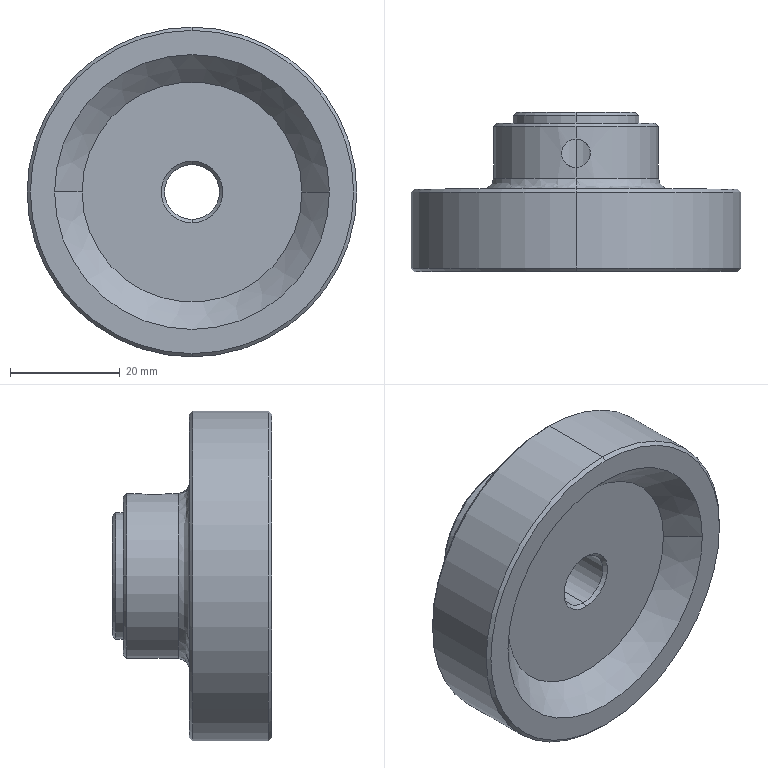Part | SolidWorks | features BaseBody 1 | 1 solid | 31 faces | box 60 x 29 x 60 mm | volume 41614 mm3 | cone 14 | cylinder 10 | plane 5 | spline 2 | commonest cylinder face diameters 5.2 x2 10 x2 23 x2 30 x2 60 x2
STEP:
#1=CARTESIAN_POINT('',(0.,10.655,-15.));
#2=VERTEX_POINT('',#1);
#3=CARTESIAN_POINT('',(0.,10.655,15.));
#4=VERTEX_POINT('',#3);
#5=CARTESIAN_POINT('',(0.,10.655,0.));
#6=DIRECTION('',(0.,1.,0.));
#7=DIRECTION('',(0.,0.,1.));
#8=AXIS2_PLACEMENT_3D('',#5,#6,#7);
#9=CIRCLE('',#8,15.);
#10=EDGE_CURVE('',#2,#4,#9,.T.);
#11=ORIENTED_EDGE('',*,*,#10,.F.);
#12=CARTESIAN_POINT('',(0.,8.655,-17.));
#13=VERTEX_POINT('',#12);
#14=CARTESIAN_POINT('',(0.,10.655,-17.));
#15=DIRECTION('',(1.,0.,0.));
#16=DIRECTION('',(0.,0.,-1.));
#17=AXIS2_PLACEMENT_3D('',#14,#15,#16);
#18=CIRCLE('',#17,2.);
#19=EDGE_CURVE('',#2,#13,#18,.T.);
#20=ORIENTED_EDGE('',*,*,#19,.T.);
#21=CARTESIAN_POINT('',(0.,8.655,17.));
#22=VERTEX_POINT('',#21);
#23=CARTESIAN_POINT('',(0.,8.655,17.));
#24=CARTESIAN_POINT('',(-0.5198,8.655,17.));
#25=CARTESIAN_POINT('',(-1.296,8.655,16.965));
#26=CARTESIAN_POINT('',(-2.197,8.655,16.861));
#27=CARTESIAN_POINT('',(-2.646,8.655,16.794));
#28=CARTESIAN_POINT('',(-2.87,8.655,16.756));
#29=CARTESIAN_POINT('',(-2.966,8.655,16.739));
#30=CARTESIAN_POINT('',(-3.029,8.655,16.728));
#31=CARTESIAN_POINT('',(-3.059,8.655,16.722));
#32=CARTESIAN_POINT('',(-3.635,8.655,16.616));
#33=CARTESIAN_POINT('',(-4.437,8.655,16.427));
#34=CARTESIAN_POINT('',(-5.354,8.655,16.139));
#35=CARTESIAN_POINT('',(-5.807,8.655,15.978));
#36=CARTESIAN_POINT('',(-6.033,8.655,15.894));
#37=CARTESIAN_POINT('',(-6.129,8.655,15.857));
#38=CARTESIAN_POINT('',(-6.193,8.655,15.832));
#39=CARTESIAN_POINT('',(-6.224,8.655,15.82));
#40=CARTESIAN_POINT('',(-6.792,8.655,15.595));
#41=CARTESIAN_POINT('',(-7.573,8.655,15.239));
#42=CARTESIAN_POINT('',(-8.449,8.655,14.757));
#43=CARTESIAN_POINT('',(-8.879,8.655,14.498));
#44=CARTESIAN_POINT('',(-9.061,8.655,14.384));
#45=CARTESIAN_POINT('',(-9.182,8.655,14.307));
#46=CARTESIAN_POINT('',(-9.241,8.655,14.269));
#47=CARTESIAN_POINT('',(-10.285,8.655,13.587));
#48=CARTESIAN_POINT('',(-11.191,8.655,12.85));
#49=CARTESIAN_POINT('',(-12.436,8.655,11.606));
#50=CARTESIAN_POINT('',(-13.023,8.655,10.955));
#51=CARTESIAN_POINT('',(-13.646,8.655,10.146));
#52=CARTESIAN_POINT('',(-13.943,8.655,9.728));
#53=CARTESIAN_POINT('',(-14.066,8.655,9.547));
#54=CARTESIAN_POINT('',(-14.148,8.655,9.425));
#55=CARTESIAN_POINT('',(-14.19,8.655,9.363));
#56=CARTESIAN_POINT('',(-14.543,8.655,8.822));
#57=CARTESIAN_POINT('',(-14.976,8.655,8.081));
#58=CARTESIAN_POINT('',(-15.414,8.655,7.181));
#59=CARTESIAN_POINT('',(-15.616,8.655,6.722));
#60=CARTESIAN_POINT('',(-15.712,8.655,6.491));
#61=CARTESIAN_POINT('',(-15.753,8.655,6.391));
#62=CARTESIAN_POINT('',(-15.78,8.655,6.324));
#63=CARTESIAN_POINT('',(-15.794,8.655,6.29));
#64=CARTESIAN_POINT('',(-16.009,8.655,5.745));
#65=CARTESIAN_POINT('',(-16.275,8.655,4.965));
#66=CARTESIAN_POINT('',(-16.518,8.655,4.036));
#67=CARTESIAN_POINT('',(-16.623,8.655,3.566));
#68=CARTESIAN_POINT('',(-16.671,8.655,3.33));
#69=CARTESIAN_POINT('',(-16.691,8.655,3.229));
#70=CARTESIAN_POINT('',(-16.704,8.655,3.161));
#71=CARTESIAN_POINT('',(-16.71,8.655,3.125));
#72=CARTESIAN_POINT('',(-16.905,8.655,2.071));
#73=CARTESIAN_POINT('',(-17.,8.655,1.039));
#74=CARTESIAN_POINT('',(-17.,8.655,-0.5197));
#75=CARTESIAN_POINT('',(-16.965,8.655,-1.296));
#76=CARTESIAN_POINT('',(-16.861,8.655,-2.197));
#77=CARTESIAN_POINT('',(-16.794,8.655,-2.645));
#78=CARTESIAN_POINT('',(-16.756,8.655,-2.87));
#79=CARTESIAN_POINT('',(-16.739,8.655,-2.965));
#80=CARTESIAN_POINT('',(-16.728,8.655,-3.029));
#81=CARTESIAN_POINT('',(-16.722,8.655,-3.059));
#82=CARTESIAN_POINT('',(-16.616,8.655,-3.635));
#83=CARTESIAN_POINT('',(-16.427,8.655,-4.437));
#84=CARTESIAN_POINT('',(-16.139,8.655,-5.354));
#85=CARTESIAN_POINT('',(-15.978,8.655,-5.807));
#86=CARTESIAN_POINT('',(-15.894,8.655,-6.033));
#87=CARTESIAN_POINT('',(-15.857,8.655,-6.129));
#88=CARTESIAN_POINT('',(-15.832,8.655,-6.193));
#89=CARTESIAN_POINT('',(-15.82,8.655,-6.224));
#90=CARTESIAN_POINT('',(-15.595,8.655,-6.792));
#91=CARTESIAN_POINT('',(-15.239,8.655,-7.573));
#92=CARTESIAN_POINT('',(-14.757,8.655,-8.449));
#93=CARTESIAN_POINT('',(-14.498,8.655,-8.879));
#94=CARTESIAN_POINT('',(-14.384,8.655,-9.061));
#95=CARTESIAN_POINT('',(-14.307,8.655,-9.182));
#96=CARTESIAN_POINT('',(-14.269,8.655,-9.241));
#97=CARTESIAN_POINT('',(-13.587,8.655,-10.285));
#98=CARTESIAN_POINT('',(-12.85,8.655,-11.191));
#99=CARTESIAN_POINT('',(-11.606,8.655,-12.436));
#100=CARTESIAN_POINT('',(-10.955,8.655,-13.023));
#101=CARTESIAN_POINT('',(-10.146,8.655,-13.646));
#102=CARTESIAN_POINT('',(-9.728,8.655,-13.943));
#103=CARTESIAN_POINT('',(-9.547,8.655,-14.066));
#104=CARTESIAN_POINT('',(-9.425,8.655,-14.148));
#105=CARTESIAN_POINT('',(-9.363,8.655,-14.19));
#106=CARTESIAN_POINT('',(-8.822,8.655,-14.543));
#107=CARTESIAN_POINT('',(-8.081,8.655,-14.976));
#108=CARTESIAN_POINT('',(-7.181,8.655,-15.414));
#109=CARTESIAN_POINT('',(-6.722,8.655,-15.616));
#110=CARTESIAN_POINT('',(-6.491,8.655,-15.712));
#111=CARTESIAN_POINT('',(-6.391,8.655,-15.753));
#112=CARTESIAN_POINT('',(-6.324,8.655,-15.78));
#113=CARTESIAN_POINT('',(-6.29,8.655,-15.794));
#114=CARTESIAN_POINT('',(-5.745,8.655,-16.009));
#115=CARTESIAN_POINT('',(-4.965,8.655,-16.275));
#116=CARTESIAN_POINT('',(-4.036,8.655,-16.518));
#117=CARTESIAN_POINT('',(-3.566,8.655,-16.623));
#118=CARTESIAN_POINT('',(-3.33,8.655,-16.671));
#119=CARTESIAN_POINT('',(-3.229,8.655,-16.691));
#120=CARTESIAN_POINT('',(-3.161,8.655,-16.704));
#121=CARTESIAN_POINT('',(-3.125,8.655,-16.71));
#122=CARTESIAN_POINT('',(-2.071,8.655,-16.905));
#123=CARTESIAN_POINT('',(-1.04,8.655,-17.));
#124=CARTESIAN_POINT('',(0.,8.655,-17.));
#125=B_SPLINE_CURVE_WITH_KNOTS('',3,(#23,#24,#25,#26,#27,#28,#29,#30,#31,#32,#33,#34,#35,#36,#37,#38,#39,#40,#41,#42,#43,#44,#45,#46,#47,#48,#49,#50,#51,#52,#53,#54,#55,#56,#57,#58,#59,#60,#61,#62,#63,#64,#65,#66,#67,#68,#69,#70,#71,#72,#73,#74,#75,#76,#77,#78,#79,#80,#81,#82,#83,#84,#85,#86,#87,#88,#89,#90,#91,#92,#93,#94,#95,#96,#97,#98,#99,#100,#101,#102,#103,#104,#105,#106,#107,#108,#109,#110,#111,#112,#113,#114,#115,#116,#117,#118,#119,#120,#121,#122,#123,#124),.UNSPECIFIED.,.F.,.F.,(4,1,1,1,1,2,2,1,1,1,1,2,2,1,1,1,2,2,2,1,1,1,2,2,1,1,1,1,2,2,1,1,1,1,2,2,2,1,1,1,1,2,2,1,1,1,1,2,2,1,1,1,2,2,2,1,1,1,2,2,1,1,1,1,2,2,1,1,1,1,2,2,4),(0.,0.03125,0.04688,0.05469,0.05859,0.06055,0.0625,0.09375,0.1094,0.1172,0.1211,0.123,0.125,0.1562,0.1719,0.1797,0.1836,0.1875,0.25,0.2812,0.2969,0.3047,0.3086,0.3125,0.3437,0.3594,0.3672,0.3711,0.373,0.375,0.4062,0.4219,0.4297,0.4336,0.4355,0.4375,0.5,0.5313,0.5469,0.5547,0.5586,0.5605,0.5625,0.5938,0.6094,0.6172,0.6211,0.623,0.625,0.6563,0.6719,0.6797,0.6836,0.6875,0.75,0.7813,0.7969,0.8047,0.8086,0.8125,0.8438,0.8594,0.8672,0.8711,0.873,0.875,0.9063,0.9219,0.9297,0.9336,0.9355,0.9375,1.),.UNSPECIFIED.);
#126=EDGE_CURVE('',#22,#13,#125,.T.);
#127=ORIENTED_EDGE('',*,*,#126,.F.);
#128=CARTESIAN_POINT('',(0.,10.655,17.));
#129=DIRECTION('',(-1.,0.,0.));
#130=DIRECTION('',(0.,0.,1.));
#131=AXIS2_PLACEMENT_3D('',#128,#129,#130);
#132=CIRCLE('',#131,2.);
#133=EDGE_CURVE('',#4,#22,#132,.T.);
#134=ORIENTED_EDGE('',*,*,#133,.F.);
#135=EDGE_LOOP('',(#11,#20,#127,#134));
#136=FACE_OUTER_BOUND('',#135,.T.);
#137=CARTESIAN_POINT('',(0.,10.655,15.));
#138=CARTESIAN_POINT('',(-30.,10.655,15.));
#139=CARTESIAN_POINT('',(-30.,10.655,-15.));
#140=CARTESIAN_POINT('',(0.,10.655,-15.));
#141=CARTESIAN_POINT('',(0.,9.484,15.));
#142=CARTESIAN_POINT('',(-30.,9.484,15.));
#143=CARTESIAN_POINT('',(-30.,9.484,-15.));
#144=CARTESIAN_POINT('',(0.,9.484,-15.));
#145=CARTESIAN_POINT('',(0.,8.655,15.828));
#146=CARTESIAN_POINT('',(-31.657,8.655,15.828));
#147=CARTESIAN_POINT('',(-31.657,8.655,-15.828));
#148=CARTESIAN_POINT('',(0.,8.655,-15.828));
#149=CARTESIAN_POINT('',(0.,8.655,17.));
#150=CARTESIAN_POINT('',(-34.,8.655,17.));
#151=CARTESIAN_POINT('',(-34.,8.655,-17.));
#152=CARTESIAN_POINT('',(0.,8.655,-17.));
#153=(BOUNDED_SURFACE()B_SPLINE_SURFACE(3,3,((#137,#138,#139,#140),(#141,#142,#143,#144),(#145,#146,#147,#148),(#149,#150,#151,#152)),.UNSPECIFIED.,.F.,.F.,.F.)B_SPLINE_SURFACE_WITH_KNOTS((4,4),(4,4),(0.,1.),(0.,1.),.UNSPECIFIED.)GEOMETRIC_REPRESENTATION_ITEM()RATIONAL_B_SPLINE_SURFACE(((1.,0.3333,0.3333,1.),(0.8047,0.2682,0.2682,0.8047),(0.8047,0.2682,0.2682,0.8047),(1.,0.3333,0.3333,1.)))REPRESENTATION_ITEM('')SURFACE());
#154=ADVANCED_FACE('',(#136),#153,.F.);
#155=CARTESIAN_POINT('',(0.,8.655,29.4));
#156=VERTEX_POINT('',#155);
#157=CARTESIAN_POINT('',(0.,8.655,-29.4));
#158=VERTEX_POINT('',#157);
#159=CARTESIAN_POINT('',(0.,8.655,0.));
#160=DIRECTION('',(0.,1.,0.));
#161=DIRECTION('',(0.,0.,-1.));
#162=AXIS2_PLACEMENT_3D('',#159,#160,#161);
#163=CIRCLE('',#162,29.4);
#164=EDGE_CURVE('',#156,#158,#163,.T.);
#165=ORIENTED_EDGE('',*,*,#164,.F.);
#166=CARTESIAN_POINT('',(0.,8.055,30.));
#167=VERTEX_POINT('',#166);
#168=CARTESIAN_POINT('',(0.,8.055,30.));
#169=DIRECTION('',(0.,-0.7071,0.7071));
#170=VECTOR('',#169,1000.);
#171=LINE('',#168,#170);
#172=EDGE_CURVE('',#156,#167,#171,.T.);
#173=ORIENTED_EDGE('',*,*,#172,.T.);
#174=CARTESIAN_POINT('',(0.,8.055,-30.));
#175=VERTEX_POINT('',#174);
#176=CARTESIAN_POINT('',(0.,8.055,0.));
#177=DIRECTION('',(0.,1.,0.));
#178=DIRECTION('',(0.,0.,1.));
#179=AXIS2_PLACEMENT_3D('',#176,#177,#178);
#180=CIRCLE('',#179,30.);
#181=EDGE_CURVE('',#167,#175,#180,.T.);
#182=ORIENTED_EDGE('',*,*,#181,.T.);
#183=CARTESIAN_POINT('',(0.,8.055,-30.));
#184=DIRECTION('',(0.,-0.7071,-0.7071));
#185=VECTOR('',#184,1000.);
#186=LINE('',#183,#185);
#187=EDGE_CURVE('',#158,#175,#186,.T.);
#188=ORIENTED_EDGE('',*,*,#187,.F.);
#189=EDGE_LOOP('',(#165,#173,#182,#188));
#190=FACE_OUTER_BOUND('',#189,.T.);
#191=CARTESIAN_POINT('',(0.,8.055,0.));
#192=DIRECTION('',(0.,-1.,0.));
#193=DIRECTION('',(0.,0.,-1.));
#194=AXIS2_PLACEMENT_3D('',#191,#192,#193);
#195=CONICAL_SURFACE('',#194,30.,0.7854);
#196=ADVANCED_FACE('',(#190),#195,.T.);
#197=CARTESIAN_POINT('',(15.,20.055,0.));
#198=VERTEX_POINT('',#197);
#199=CARTESIAN_POINT('',(0.,20.055,15.));
#200=VERTEX_POINT('',#199);
#201=CARTESIAN_POINT('',(0.,20.055,0.));
#202=DIRECTION('',(0.,-1.,0.));
#203=DIRECTION('',(0.,0.,-1.));
#204=AXIS2_PLACEMENT_3D('',#201,#202,#203);
#205=CIRCLE('',#204,15.);
#206=EDGE_CURVE('',#198,#200,#205,.T.);
#207=ORIENTED_EDGE('',*,*,#206,.T.);
#208=CARTESIAN_POINT('',(0.,17.755,15.));
#209=VERTEX_POINT('',#208);
#210=CARTESIAN_POINT('',(0.,0.,15.));
#211=DIRECTION('',(0.,-1.,0.));
#212=VECTOR('',#211,1000.);
#213=LINE('',#210,#212);
#214=EDGE_CURVE('',#200,#209,#213,.T.);
#215=ORIENTED_EDGE('',*,*,#214,.T.);
#216=CARTESIAN_POINT('',(2.6,15.155,14.773));
#217=VERTEX_POINT('',#216);
#218=CARTESIAN_POINT('',(0.,17.755,15.));
#219=CARTESIAN_POINT('',(0.172,17.755,15.));
#220=CARTESIAN_POINT('',(0.3411,17.739,14.997));
#221=CARTESIAN_POINT('',(0.6737,17.672,14.986));
#222=CARTESIAN_POINT('',(0.8389,17.622,14.977));
#223=CARTESIAN_POINT('',(1.153,17.492,14.956));
#224=CARTESIAN_POINT('',(1.303,17.412,14.944));
#225=CARTESIAN_POINT('',(1.585,17.224,14.917));
#226=CARTESIAN_POINT('',(1.718,17.114,14.902));
#227=CARTESIAN_POINT('',(1.958,16.875,14.872));
#228=CARTESIAN_POINT('',(2.065,16.744,14.857));
#229=CARTESIAN_POINT('',(2.255,16.461,14.83));
#230=CARTESIAN_POINT('',(2.336,16.31,14.817));
#231=CARTESIAN_POINT('',(2.531,15.841,14.786));
#232=CARTESIAN_POINT('',(2.6,15.5,14.773));
#233=CARTESIAN_POINT('',(2.6,15.155,14.773));
#234=B_SPLINE_CURVE_WITH_KNOTS('',3,(#218,#219,#220,#221,#222,#223,#224,#225,#226,#227,#228,#229,#230,#231,#232,#233),.UNSPECIFIED.,.F.,.F.,(4,2,2,2,2,2,2,4),(0.004069,0.004578,0.005087,0.005595,0.006104,0.006613,0.007121,0.008139),.UNSPECIFIED.);
#235=EDGE_CURVE('',#209,#217,#234,.T.);
#236=ORIENTED_EDGE('',*,*,#235,.T.);
#237=CARTESIAN_POINT('',(0.,12.555,15.));
#238=VERTEX_POINT('',#237);
#239=CARTESIAN_POINT('',(2.6,15.155,14.773));
#240=CARTESIAN_POINT('',(2.6,14.983,14.773));
#241=CARTESIAN_POINT('',(2.583,14.814,14.776));
#242=CARTESIAN_POINT('',(2.517,14.482,14.787));
#243=CARTESIAN_POINT('',(2.467,14.317,14.796));
#244=CARTESIAN_POINT('',(2.336,14.002,14.817));
#245=CARTESIAN_POINT('',(2.257,13.853,14.83));
#246=CARTESIAN_POINT('',(2.068,13.571,14.857));
#247=CARTESIAN_POINT('',(1.959,13.437,14.872));
#248=CARTESIAN_POINT('',(1.719,13.198,14.902));
#249=CARTESIAN_POINT('',(1.589,13.09,14.916));
#250=CARTESIAN_POINT('',(1.305,12.9,14.944));
#251=CARTESIAN_POINT('',(1.154,12.82,14.956));
#252=CARTESIAN_POINT('',(0.6858,12.625,14.988));
#253=CARTESIAN_POINT('',(0.344,12.555,15.));
#254=CARTESIAN_POINT('',(0.,12.555,15.));
#255=B_SPLINE_CURVE_WITH_KNOTS('',3,(#239,#240,#241,#242,#243,#244,#245,#246,#247,#248,#249,#250,#251,#252,#253,#254),.UNSPECIFIED.,.F.,.F.,(4,2,2,2,2,2,2,4),(-0.008138,-0.00763,-0.007121,-0.006612,-0.006104,-0.005595,-0.005087,-0.004069),.UNSPECIFIED.);
#256=EDGE_CURVE('',#217,#238,#255,.T.);
#257=ORIENTED_EDGE('',*,*,#256,.T.);
#258=CARTESIAN_POINT('',(0.,0.,15.));
#259=DIRECTION('',(0.,-1.,0.));
#260=VECTOR('',#259,1000.);
#261=LINE('',#258,#260);
#262=EDGE_CURVE('',#238,#4,#261,.T.);
#263=ORIENTED_EDGE('',*,*,#262,.T.);
#264=CARTESIAN_POINT('',(0.,10.655,0.));
#265=DIRECTION('',(0.,1.,0.));
#266=DIRECTION('',(0.,0.,1.));
#267=AXIS2_PLACEMENT_3D('',#264,#265,#266);
#268=CIRCLE('',#267,15.);
#269=EDGE_CURVE('',#4,#2,#268,.T.);
#270=ORIENTED_EDGE('',*,*,#269,.T.);
#271=CARTESIAN_POINT('',(0.,20.055,-15.));
#272=VERTEX_POINT('',#271);
#273=CARTESIAN_POINT('',(0.,0.,-15.));
#274=DIRECTION('',(0.,-1.,0.));
#275=VECTOR('',#274,1000.);
#276=LINE('',#273,#275);
#277=EDGE_CURVE('',#272,#2,#276,.T.);
#278=ORIENTED_EDGE('',*,*,#277,.F.);
#279=CARTESIAN_POINT('',(0.,20.055,0.));
#280=DIRECTION('',(0.,-1.,0.));
#281=DIRECTION('',(0.,0.,-1.));
#282=AXIS2_PLACEMENT_3D('',#279,#280,#281);
#283=CIRCLE('',#282,15.);
#284=EDGE_CURVE('',#272,#198,#283,.T.);
#285=ORIENTED_EDGE('',*,*,#284,.T.);
#286=EDGE_LOOP('',(#207,#215,#236,#257,#263,#270,#278,#285));
#287=FACE_OUTER_BOUND('',#286,.T.);
#288=CARTESIAN_POINT('',(0.,0.,0.));
#289=DIRECTION('',(0.,-1.,0.));
#290=DIRECTION('',(0.,0.,-1.));
#291=AXIS2_PLACEMENT_3D('',#288,#289,#290);
#292=CYLINDRICAL_SURFACE('',#291,15.);
#293=ADVANCED_FACE('',(#287),#292,.T.);
#294=ORIENTED_EDGE('',*,*,#181,.F.);
#295=CARTESIAN_POINT('',(0.,-5.745,30.));
#296=VERTEX_POINT('',#295);
#297=CARTESIAN_POINT('',(0.,0.,30.));
#298=DIRECTION('',(0.,-1.,0.));
#299=VECTOR('',#298,1000.);
#300=LINE('',#297,#299);
#301=EDGE_CURVE('',#167,#296,#300,.T.);
#302=ORIENTED_EDGE('',*,*,#301,.T.);
#303=CARTESIAN_POINT('',(0.,-5.745,-30.));
#304=VERTEX_POINT('',#303);
#305=CARTESIAN_POINT('',(0.,-5.745,0.));
#306=DIRECTION('',(0.,1.,0.));
#307=DIRECTION('',(0.,0.,-1.));
#308=AXIS2_PLACEMENT_3D('',#305,#306,#307);
#309=CIRCLE('',#308,30.);
#310=EDGE_CURVE('',#296,#304,#309,.T.);
#311=ORIENTED_EDGE('',*,*,#310,.T.);
#312=CARTESIAN_POINT('',(0.,0.,-30.));
#313=DIRECTION('',(0.,-1.,0.));
#314=VECTOR('',#313,1000.);
#315=LINE('',#312,#314);
#316=EDGE_CURVE('',#175,#304,#315,.T.);
#317=ORIENTED_EDGE('',*,*,#316,.F.);
#318=EDGE_LOOP('',(#294,#302,#311,#317));
#319=FACE_OUTER_BOUND('',#318,.T.);
#320=CARTESIAN_POINT('',(0.,0.,0.));
#321=DIRECTION('',(0.,-1.,0.));
#322=DIRECTION('',(0.,0.,-1.));
#323=AXIS2_PLACEMENT_3D('',#320,#321,#322);
#324=CYLINDRICAL_SURFACE('',#323,30.);
#325=ADVANCED_FACE('',(#319),#324,.T.);
#326=ORIENTED_EDGE('',*,*,#256,.F.);
#327=CARTESIAN_POINT('',(2.6,15.155,4.271));
#328=VERTEX_POINT('',#327);
#329=CARTESIAN_POINT('',(2.6,15.155,30.));
#330=DIRECTION('',(0.,0.,-1.));
#331=VECTOR('',#330,1000.);
#332=LINE('',#329,#331);
#333=EDGE_CURVE('',#217,#328,#332,.T.);
#334=ORIENTED_EDGE('',*,*,#333,.T.);
#335=CARTESIAN_POINT('',(0.,12.555,5.));
#336=VERTEX_POINT('',#335);
#337=CARTESIAN_POINT('',(0.,12.555,5.));
#338=CARTESIAN_POINT('',(0.1752,12.555,5.));
#339=CARTESIAN_POINT('',(0.3469,12.573,4.991));
#340=CARTESIAN_POINT('',(0.6838,12.641,4.956));
#341=CARTESIAN_POINT('',(0.8506,12.693,4.93));
#342=CARTESIAN_POINT('',(1.321,12.891,4.833));
#343=CARTESIAN_POINT('',(1.605,13.083,4.742));
#344=CARTESIAN_POINT('',(1.958,13.437,4.602));
#345=CARTESIAN_POINT('',(2.065,13.567,4.555));
#346=CARTESIAN_POINT('',(2.252,13.846,4.465));
#347=CARTESIAN_POINT('',(2.332,13.993,4.424));
#348=CARTESIAN_POINT('',(2.462,14.304,4.352));
#349=CARTESIAN_POINT('',(2.514,14.47,4.322));
#350=CARTESIAN_POINT('',(2.582,14.808,4.282));
#351=CARTESIAN_POINT('',(2.6,14.98,4.271));
#352=CARTESIAN_POINT('',(2.6,15.155,4.271));
#353=B_SPLINE_CURVE_WITH_KNOTS('',3,(#337,#338,#339,#340,#341,#342,#343,#344,#345,#346,#347,#348,#349,#350,#351,#352),.UNSPECIFIED.,.F.,.F.,(4,2,2,2,2,2,2,4),(0.00828,0.008797,0.009315,0.01035,0.01087,0.01138,0.0119,0.01242),.UNSPECIFIED.);
#354=EDGE_CURVE('',#336,#328,#353,.T.);
#355=ORIENTED_EDGE('',*,*,#354,.F.);
#356=CARTESIAN_POINT('',(-2.6,15.155,4.271));
#357=VERTEX_POINT('',#356);
#358=CARTESIAN_POINT('',(-2.6,15.155,4.271));
#359=CARTESIAN_POINT('',(-2.6,14.98,4.271));
#360=CARTESIAN_POINT('',(-2.582,14.809,4.282));
#361=CARTESIAN_POINT('',(-2.515,14.472,4.322));
#362=CARTESIAN_POINT('',(-2.463,14.306,4.352));
#363=CARTESIAN_POINT('',(-2.266,13.837,4.459));
#364=CARTESIAN_POINT('',(-2.075,13.554,4.556));
#365=CARTESIAN_POINT('',(-1.722,13.201,4.696));
#366=CARTESIAN_POINT('',(-1.592,13.093,4.742));
#367=CARTESIAN_POINT('',(-1.313,12.905,4.827));
#368=CARTESIAN_POINT('',(-1.165,12.825,4.865));
#369=CARTESIAN_POINT('',(-0.8525,12.693,4.929));
#370=CARTESIAN_POINT('',(-0.6858,12.642,4.956));
#371=CARTESIAN_POINT('',(-0.3474,12.573,4.991));
#372=CARTESIAN_POINT('',(-0.1753,12.555,5.));
#373=CARTESIAN_POINT('',(0.,12.555,5.));
#374=B_SPLINE_CURVE_WITH_KNOTS('',3,(#358,#359,#360,#361,#362,#363,#364,#365,#366,#367,#368,#369,#370,#371,#372,#373),.UNSPECIFIED.,.F.,.F.,(4,2,2,2,2,2,2,4),(0.004141,0.004658,0.005175,0.00621,0.006728,0.007245,0.007763,0.00828),.UNSPECIFIED.);
#375=EDGE_CURVE('',#357,#336,#374,.T.);
#376=ORIENTED_EDGE('',*,*,#375,.F.);
#377=CARTESIAN_POINT('',(-2.6,15.155,14.773));
#378=VERTEX_POINT('',#377);
#379=CARTESIAN_POINT('',(-2.6,15.155,30.));
#380=DIRECTION('',(0.,0.,-1.));
#381=VECTOR('',#380,1000.);
#382=LINE('',#379,#381);
#383=EDGE_CURVE('',#378,#357,#382,.T.);
#384=ORIENTED_EDGE('',*,*,#383,.F.);
#385=CARTESIAN_POINT('',(0.,12.555,15.));
#386=CARTESIAN_POINT('',(-0.172,12.555,15.));
#387=CARTESIAN_POINT('',(-0.3411,12.572,14.997));
#388=CARTESIAN_POINT('',(-0.6737,12.639,14.986));
#389=CARTESIAN_POINT('',(-0.8389,12.689,14.977));
#390=CARTESIAN_POINT('',(-1.153,12.819,14.956));
#391=CARTESIAN_POINT('',(-1.303,12.899,14.944));
#392=CARTESIAN_POINT('',(-1.585,13.087,14.917));
#393=CARTESIAN_POINT('',(-1.718,13.197,14.902));
#394=CARTESIAN_POINT('',(-1.958,13.436,14.872));
#395=CARTESIAN_POINT('',(-2.065,13.567,14.857));
#396=CARTESIAN_POINT('',(-2.255,13.85,14.83));
#397=CARTESIAN_POINT('',(-2.336,14.001,14.817));
#398=CARTESIAN_POINT('',(-2.531,14.47,14.786));
#399=CARTESIAN_POINT('',(-2.6,14.811,14.773));
#400=CARTESIAN_POINT('',(-2.6,15.155,14.773));
#401=B_SPLINE_CURVE_WITH_KNOTS('',3,(#385,#386,#387,#388,#389,#390,#391,#392,#393,#394,#395,#396,#397,#398,#399,#400),.UNSPECIFIED.,.F.,.F.,(4,2,2,2,2,2,2,4),(-0.004069,-0.003561,-0.003052,-0.002543,-0.002035,-0.001526,-0.001017,0.),.UNSPECIFIED.);
#402=EDGE_CURVE('',#238,#378,#401,.T.);
#403=ORIENTED_EDGE('',*,*,#402,.F.);
#404=EDGE_LOOP('',(#326,#334,#355,#376,#384,#403));
#405=FACE_OUTER_BOUND('',#404,.T.);
#406=CARTESIAN_POINT('',(0.,15.155,30.));
#407=DIRECTION('',(0.,0.,-1.));
#408=DIRECTION('',(-1.,0.,0.));
#409=AXIS2_PLACEMENT_3D('',#406,#407,#408);
#410=CYLINDRICAL_SURFACE('',#409,2.6);
#411=ADVANCED_FACE('',(#405),#410,.F.);
#412=CARTESIAN_POINT('',(14.4,20.655,0.));
#413=VERTEX_POINT('',#412);
#414=CARTESIAN_POINT('',(-14.4,20.655,0.));
#415=VERTEX_POINT('',#414);
#416=CARTESIAN_POINT('',(0.,20.655,0.));
#417=DIRECTION('',(0.,-1.,0.));
#418=DIRECTION('',(1.,0.,0.));
#419=AXIS2_PLACEMENT_3D('',#416,#417,#418);
#420=CIRCLE('',#419,14.4);
#421=EDGE_CURVE('',#413,#415,#420,.T.);
#422=ORIENTED_EDGE('',*,*,#421,.T.);
#423=CARTESIAN_POINT('',(-15.,20.055,0.));
#424=VERTEX_POINT('',#423);
#425=CARTESIAN_POINT('',(-15.,20.055,0.));
#426=DIRECTION('',(-0.7071,-0.7071,0.));
#427=VECTOR('',#426,1000.);
#428=LINE('',#425,#427);
#429=EDGE_CURVE('',#415,#424,#428,.T.);
#430=ORIENTED_EDGE('',*,*,#429,.T.);
#431=CARTESIAN_POINT('',(0.,20.055,0.));
#432=DIRECTION('',(0.,-1.,0.));
#433=DIRECTION('',(0.,0.,-1.));
#434=AXIS2_PLACEMENT_3D('',#431,#432,#433);
#435=CIRCLE('',#434,15.);
#436=EDGE_CURVE('',#200,#424,#435,.T.);
#437=ORIENTED_EDGE('',*,*,#436,.F.);
#438=ORIENTED_EDGE('',*,*,#206,.F.);
#439=CARTESIAN_POINT('',(15.,20.055,0.));
#440=DIRECTION('',(0.7071,-0.7071,0.));
#441=VECTOR('',#440,1000.);
#442=LINE('',#439,#441);
#443=EDGE_CURVE('',#413,#198,#442,.T.);
#444=ORIENTED_EDGE('',*,*,#443,.F.);
#445=EDGE_LOOP('',(#422,#430,#437,#438,#444));
#446=FACE_OUTER_BOUND('',#445,.T.);
#447=CARTESIAN_POINT('',(0.,20.055,0.));
#448=DIRECTION('',(0.,-1.,0.));
#449=DIRECTION('',(1.,0.,0.));
#450=AXIS2_PLACEMENT_3D('',#447,#448,#449);
#451=CONICAL_SURFACE('',#450,15.,0.7854);
#452=ADVANCED_FACE('',(#446),#451,.T.);
#453=CARTESIAN_POINT('',(0.,-6.345,29.4));
#454=VERTEX_POINT('',#453);
#455=CARTESIAN_POINT('',(0.,-6.345,-29.4));
#456=VERTEX_POINT('',#455);
#457=CARTESIAN_POINT('',(0.,-6.345,0.));
#458=DIRECTION('',(0.,1.,0.));
#459=DIRECTION('',(0.,0.,1.));
#460=AXIS2_PLACEMENT_3D('',#457,#458,#459);
#461=CIRCLE('',#460,29.4);
#462=EDGE_CURVE('',#454,#456,#461,.T.);
#463=ORIENTED_EDGE('',*,*,#462,.T.);
#464=CARTESIAN_POINT('',(0.,-5.745,-30.));
#465=DIRECTION('',(0.,0.7071,-0.7071));
#466=VECTOR('',#465,1000.);
#467=LINE('',#464,#466);
#468=EDGE_CURVE('',#456,#304,#467,.T.);
#469=ORIENTED_EDGE('',*,*,#468,.T.);
#470=ORIENTED_EDGE('',*,*,#310,.F.);
#471=CARTESIAN_POINT('',(0.,-5.745,30.));
#472=DIRECTION('',(0.,0.7071,0.7071));
#473=VECTOR('',#472,1000.);
#474=LINE('',#471,#473);
#475=EDGE_CURVE('',#454,#296,#474,.T.);
#476=ORIENTED_EDGE('',*,*,#475,.F.);
#477=EDGE_LOOP('',(#463,#469,#470,#476));
#478=FACE_OUTER_BOUND('',#477,.T.);
#479=CARTESIAN_POINT('',(0.,-5.745,0.));
#480=DIRECTION('',(0.,1.,0.));
#481=DIRECTION('',(0.,0.,1.));
#482=AXIS2_PLACEMENT_3D('',#479,#480,#481);
#483=CONICAL_SURFACE('',#482,30.,0.7854);
#484=ADVANCED_FACE('',(#478),#483,.T.);
#485=CARTESIAN_POINT('',(0.,22.055,5.));
#486=VERTEX_POINT('',#485);
#487=CARTESIAN_POINT('',(0.,22.055,-5.));
#488=VERTEX_POINT('',#487);
#489=CARTESIAN_POINT('',(0.,22.055,0.));
#490=DIRECTION('',(0.,-1.,0.));
#491=DIRECTION('',(0.,0.,-1.));
#492=AXIS2_PLACEMENT_3D('',#489,#490,#491);
#493=CIRCLE('',#492,5.);
#494=EDGE_CURVE('',#486,#488,#493,.T.);
#495=ORIENTED_EDGE('',*,*,#494,.F.);
#496=CARTESIAN_POINT('',(0.,17.755,5.));
#497=VERTEX_POINT('',#496);
#498=CARTESIAN_POINT('',(0.,0.,5.));
#499=DIRECTION('',(0.,-1.,0.));
#500=VECTOR('',#499,1000.);
#501=LINE('',#498,#500);
#502=EDGE_CURVE('',#486,#497,#501,.T.);
#503=ORIENTED_EDGE('',*,*,#502,.T.);
#504=CARTESIAN_POINT('',(0.,17.755,5.));
#505=CARTESIAN_POINT('',(-0.1752,17.755,5.));
#506=CARTESIAN_POINT('',(-0.3469,17.738,4.991));
#507=CARTESIAN_POINT('',(-0.6838,17.67,4.956));
#508=CARTESIAN_POINT('',(-0.8506,17.618,4.93));
#509=CARTESIAN_POINT('',(-1.321,17.42,4.833));
#510=CARTESIAN_POINT('',(-1.605,17.228,4.742));
#511=CARTESIAN_POINT('',(-1.958,16.874,4.602));
#512=CARTESIAN_POINT('',(-2.065,16.744,4.555));
#513=CARTESIAN_POINT('',(-2.252,16.465,4.465));
#514=CARTESIAN_POINT('',(-2.332,16.318,4.424));
#515=CARTESIAN_POINT('',(-2.462,16.007,4.352));
#516=CARTESIAN_POINT('',(-2.514,15.841,4.322));
#517=CARTESIAN_POINT('',(-2.582,15.503,4.282));
#518=CARTESIAN_POINT('',(-2.6,15.331,4.271));
#519=CARTESIAN_POINT('',(-2.6,15.155,4.271));
#520=B_SPLINE_CURVE_WITH_KNOTS('',3,(#504,#505,#506,#507,#508,#509,#510,#511,#512,#513,#514,#515,#516,#517,#518,#519),.UNSPECIFIED.,.F.,.F.,(4,2,2,2,2,2,2,4),(0.,0.0005176,0.001035,0.00207,0.002588,0.003105,0.003623,0.004141),.UNSPECIFIED.);
#521=EDGE_CURVE('',#497,#357,#520,.T.);
#522=ORIENTED_EDGE('',*,*,#521,.T.);
#523=ORIENTED_EDGE('',*,*,#375,.T.);
#524=CARTESIAN_POINT('',(0.,-0.7445,5.));
#525=VERTEX_POINT('',#524);
#526=CARTESIAN_POINT('',(0.,0.,5.));
#527=DIRECTION('',(0.,-1.,0.));
#528=VECTOR('',#527,1000.);
#529=LINE('',#526,#528);
#530=EDGE_CURVE('',#336,#525,#529,.T.);
#531=ORIENTED_EDGE('',*,*,#530,.T.);
#532=CARTESIAN_POINT('',(0.,-0.7445,-5.));
#533=VERTEX_POINT('',#532);
#534=CARTESIAN_POINT('',(0.,-0.7445,0.));
#535=DIRECTION('',(0.,1.,0.));
#536=DIRECTION('',(0.,0.,-1.));
#537=AXIS2_PLACEMENT_3D('',#534,#535,#536);
#538=CIRCLE('',#537,5.);
#539=EDGE_CURVE('',#533,#525,#538,.T.);
#540=ORIENTED_EDGE('',*,*,#539,.F.);
#541=CARTESIAN_POINT('',(0.,0.,-5.));
#542=DIRECTION('',(0.,-1.,0.));
#543=VECTOR('',#542,1000.);
#544=LINE('',#541,#543);
#545=EDGE_CURVE('',#488,#533,#544,.T.);
#546=ORIENTED_EDGE('',*,*,#545,.F.);
#547=EDGE_LOOP('',(#495,#503,#522,#523,#531,#540,#546));
#548=FACE_OUTER_BOUND('',#547,.T.);
#549=CARTESIAN_POINT('',(0.,0.,0.));
#550=DIRECTION('',(0.,-1.,0.));
#551=DIRECTION('',(0.,0.,-1.));
#552=AXIS2_PLACEMENT_3D('',#549,#550,#551);
#553=CYLINDRICAL_SURFACE('',#552,5.);
#554=ADVANCED_FACE('',(#548),#553,.F.);
#555=ORIENTED_EDGE('',*,*,#494,.T.);
#556=CARTESIAN_POINT('',(0.,22.655,-5.6));
#557=VERTEX_POINT('',#556);
#558=CARTESIAN_POINT('',(0.,22.655,-5.6));
#559=DIRECTION('',(0.,0.7071,-0.7071));
#560=VECTOR('',#559,1000.);
#561=LINE('',#558,#560);
#562=EDGE_CURVE('',#488,#557,#561,.T.);
#563=ORIENTED_EDGE('',*,*,#562,.T.);
#564=CARTESIAN_POINT('',(0.,22.655,5.6));
#565=VERTEX_POINT('',#564);
#566=CARTESIAN_POINT('',(0.,22.655,0.));
#567=DIRECTION('',(0.,-1.,0.));
#568=DIRECTION('',(0.,0.,1.));
#569=AXIS2_PLACEMENT_3D('',#566,#567,#568);
#570=CIRCLE('',#569,5.6);
#571=EDGE_CURVE('',#565,#557,#570,.T.);
#572=ORIENTED_EDGE('',*,*,#571,.F.);
#573=CARTESIAN_POINT('',(0.,22.655,5.6));
#574=DIRECTION('',(0.,0.7071,0.7071));
#575=VECTOR('',#574,1000.);
#576=LINE('',#573,#575);
#577=EDGE_CURVE('',#486,#565,#576,.T.);
#578=ORIENTED_EDGE('',*,*,#577,.F.);
#579=EDGE_LOOP('',(#555,#563,#572,#578));
#580=FACE_OUTER_BOUND('',#579,.T.);
#581=CARTESIAN_POINT('',(0.,22.655,0.));
#582=DIRECTION('',(0.,1.,0.));
#583=DIRECTION('',(0.,0.,1.));
#584=AXIS2_PLACEMENT_3D('',#581,#582,#583);
#585=CONICAL_SURFACE('',#584,5.6,0.7854);
#586=ADVANCED_FACE('',(#580),#585,.F.);
#587=ORIENTED_EDGE('',*,*,#539,.T.);
#588=CARTESIAN_POINT('',(0.,-1.345,5.6));
#589=VERTEX_POINT('',#588);
#590=CARTESIAN_POINT('',(0.,-1.345,5.6));
#591=DIRECTION('',(0.,-0.7071,0.7071));
#592=VECTOR('',#591,1000.);
#593=LINE('',#590,#592);
#594=EDGE_CURVE('',#525,#589,#593,.T.);
#595=ORIENTED_EDGE('',*,*,#594,.T.);
#596=CARTESIAN_POINT('',(0.,-1.345,-5.6));
#597=VERTEX_POINT('',#596);
#598=CARTESIAN_POINT('',(0.,-1.345,0.));
#599=DIRECTION('',(0.,1.,0.));
#600=DIRECTION('',(0.,0.,-1.));
#601=AXIS2_PLACEMENT_3D('',#598,#599,#600);
#602=CIRCLE('',#601,5.6);
#603=EDGE_CURVE('',#597,#589,#602,.T.);
#604=ORIENTED_EDGE('',*,*,#603,.F.);
#605=CARTESIAN_POINT('',(0.,-1.345,-5.6));
#606=DIRECTION('',(0.,-0.7071,-0.7071));
#607=VECTOR('',#606,1000.);
#608=LINE('',#605,#607);
#609=EDGE_CURVE('',#533,#597,#608,.T.);
#610=ORIENTED_EDGE('',*,*,#609,.F.);
#611=EDGE_LOOP('',(#587,#595,#604,#610));
#612=FACE_OUTER_BOUND('',#611,.T.);
#613=CARTESIAN_POINT('',(0.,-1.345,0.));
#614=DIRECTION('',(0.,-1.,0.));
#615=DIRECTION('',(0.,0.,-1.));
#616=AXIS2_PLACEMENT_3D('',#613,#614,#615);
#617=CONICAL_SURFACE('',#616,5.6,0.7854);
#618=ADVANCED_FACE('',(#612),#617,.F.);
#619=CARTESIAN_POINT('',(0.,22.055,-11.5));
#620=VERTEX_POINT('',#619);
#621=CARTESIAN_POINT('',(0.,22.055,11.5));
#622=VERTEX_POINT('',#621);
#623=CARTESIAN_POINT('',(0.,22.055,0.));
#624=DIRECTION('',(0.,-1.,0.));
#625=DIRECTION('',(0.,0.,-1.));
#626=AXIS2_PLACEMENT_3D('',#623,#624,#625);
#627=CIRCLE('',#626,11.5);
#628=EDGE_CURVE('',#620,#622,#627,.T.);
#629=ORIENTED_EDGE('',*,*,#628,.T.);
#630=CARTESIAN_POINT('',(0.,20.655,11.5));
#631=VERTEX_POINT('',#630);
#632=CARTESIAN_POINT('',(0.,0.,11.5));
#633=DIRECTION('',(0.,-1.,0.));
#634=VECTOR('',#633,1000.);
#635=LINE('',#632,#634);
#636=EDGE_CURVE('',#622,#631,#635,.T.);
#637=ORIENTED_EDGE('',*,*,#636,.T.);
#638=CARTESIAN_POINT('',(0.,20.655,-11.5));
#639=VERTEX_POINT('',#638);
#640=CARTESIAN_POINT('',(0.,20.655,0.));
#641=DIRECTION('',(0.,1.,0.));
#642=DIRECTION('',(0.,0.,-1.));
#643=AXIS2_PLACEMENT_3D('',#640,#641,#642);
#644=CIRCLE('',#643,11.5);
#645=EDGE_CURVE('',#631,#639,#644,.T.);
#646=ORIENTED_EDGE('',*,*,#645,.T.);
#647=CARTESIAN_POINT('',(0.,0.,-11.5));
#648=DIRECTION('',(0.,-1.,0.));
#649=VECTOR('',#648,1000.);
#650=LINE('',#647,#649);
#651=EDGE_CURVE('',#620,#639,#650,.T.);
#652=ORIENTED_EDGE('',*,*,#651,.F.);
#653=EDGE_LOOP('',(#629,#637,#646,#652));
#654=FACE_OUTER_BOUND('',#653,.T.);
#655=CARTESIAN_POINT('',(0.,0.,0.));
#656=DIRECTION('',(0.,-1.,0.));
#657=DIRECTION('',(0.,0.,-1.));
#658=AXIS2_PLACEMENT_3D('',#655,#656,#657);
#659=CYLINDRICAL_SURFACE('',#658,11.5);
#660=ADVANCED_FACE('',(#654),#659,.T.);
#661=CARTESIAN_POINT('',(-20.,-1.345,0.));
#662=VERTEX_POINT('',#661);
#663=CARTESIAN_POINT('',(20.,-1.345,0.));
#664=VERTEX_POINT('',#663);
#665=CARTESIAN_POINT('',(0.,-1.345,0.));
#666=DIRECTION('',(0.,-1.,0.));
#667=DIRECTION('',(1.,0.,0.));
#668=AXIS2_PLACEMENT_3D('',#665,#666,#667);
#669=CIRCLE('',#668,20.);
#670=EDGE_CURVE('',#662,#664,#669,.T.);
#671=ORIENTED_EDGE('',*,*,#670,.F.);
#672=CARTESIAN_POINT('',(-25.,-6.345,0.));
#673=VERTEX_POINT('',#672);
#674=CARTESIAN_POINT('',(-25.,-6.345,0.));
#675=DIRECTION('',(-0.7071,-0.7071,0.));
#676=VECTOR('',#675,1000.);
#677=LINE('',#674,#676);
#678=EDGE_CURVE('',#662,#673,#677,.T.);
#679=ORIENTED_EDGE('',*,*,#678,.T.);
#680=CARTESIAN_POINT('',(25.,-6.345,0.));
#681=VERTEX_POINT('',#680);
#682=CARTESIAN_POINT('',(0.,-6.345,0.));
#683=DIRECTION('',(0.,1.,0.));
#684=DIRECTION('',(1.,0.,0.));
#685=AXIS2_PLACEMENT_3D('',#682,#683,#684);
#686=CIRCLE('',#685,25.);
#687=EDGE_CURVE('',#681,#673,#686,.T.);
#688=ORIENTED_EDGE('',*,*,#687,.F.);
#689=CARTESIAN_POINT('',(25.,-6.345,0.));
#690=DIRECTION('',(0.7071,-0.7071,0.));
#691=VECTOR('',#690,1000.);
#692=LINE('',#689,#691);
#693=EDGE_CURVE('',#664,#681,#692,.T.);
#694=ORIENTED_EDGE('',*,*,#693,.F.);
#695=EDGE_LOOP('',(#671,#679,#688,#694));
#696=FACE_OUTER_BOUND('',#695,.T.);
#697=CARTESIAN_POINT('',(0.,-6.345,0.));
#698=DIRECTION('',(0.,-1.,0.));
#699=DIRECTION('',(1.,0.,0.));
#700=AXIS2_PLACEMENT_3D('',#697,#698,#699);
#701=CONICAL_SURFACE('',#700,25.,0.7854);
#702=ADVANCED_FACE('',(#696),#701,.F.);
#703=CARTESIAN_POINT('',(0.,22.655,10.9));
#704=VERTEX_POINT('',#703);
#705=CARTESIAN_POINT('',(0.,22.655,-10.9));
#706=VERTEX_POINT('',#705);
#707=CARTESIAN_POINT('',(0.,22.655,0.));
#708=DIRECTION('',(0.,1.,0.));
#709=DIRECTION('',(0.,0.,-1.));
#710=AXIS2_PLACEMENT_3D('',#707,#708,#709);
#711=CIRCLE('',#710,10.9);
#712=EDGE_CURVE('',#704,#706,#711,.T.);
#713=ORIENTED_EDGE('',*,*,#712,.F.);
#714=CARTESIAN_POINT('',(0.,22.055,11.5));
#715=DIRECTION('',(0.,-0.7071,0.7071));
#716=VECTOR('',#715,1000.);
#717=LINE('',#714,#716);
#718=EDGE_CURVE('',#704,#622,#717,.T.);
#719=ORIENTED_EDGE('',*,*,#718,.T.);
#720=ORIENTED_EDGE('',*,*,#628,.F.);
#721=CARTESIAN_POINT('',(0.,22.055,-11.5));
#722=DIRECTION('',(0.,-0.7071,-0.7071));
#723=VECTOR('',#722,1000.);
#724=LINE('',#721,#723);
#725=EDGE_CURVE('',#706,#620,#724,.T.);
#726=ORIENTED_EDGE('',*,*,#725,.F.);
#727=EDGE_LOOP('',(#713,#719,#720,#726));
#728=FACE_OUTER_BOUND('',#727,.T.);
#729=CARTESIAN_POINT('',(0.,22.055,0.));
#730=DIRECTION('',(0.,-1.,0.));
#731=DIRECTION('',(0.,0.,-1.));
#732=AXIS2_PLACEMENT_3D('',#729,#730,#731);
#733=CONICAL_SURFACE('',#732,11.5,0.7854);
#734=ADVANCED_FACE('',(#728),#733,.T.);
#735=CARTESIAN_POINT('',(0.,8.655,-17.));
#736=CARTESIAN_POINT('',(0.5198,8.655,-17.));
#737=CARTESIAN_POINT('',(1.296,8.655,-16.965));
#738=CARTESIAN_POINT('',(2.197,8.655,-16.861));
#739=CARTESIAN_POINT('',(2.646,8.655,-16.794));
#740=CARTESIAN_POINT('',(2.87,8.655,-16.756));
#741=CARTESIAN_POINT('',(2.966,8.655,-16.739));
#742=CARTESIAN_POINT('',(3.029,8.655,-16.728));
#743=CARTESIAN_POINT('',(3.059,8.655,-16.722));
#744=CARTESIAN_POINT('',(3.635,8.655,-16.616));
#745=CARTESIAN_POINT('',(4.437,8.655,-16.427));
#746=CARTESIAN_POINT('',(5.354,8.655,-16.139));
#747=CARTESIAN_POINT('',(5.807,8.655,-15.978));
#748=CARTESIAN_POINT('',(6.033,8.655,-15.894));
#749=CARTESIAN_POINT('',(6.129,8.655,-15.857));
#750=CARTESIAN_POINT('',(6.193,8.655,-15.832));
#751=CARTESIAN_POINT('',(6.224,8.655,-15.82));
#752=CARTESIAN_POINT('',(6.792,8.655,-15.595));
#753=CARTESIAN_POINT('',(7.573,8.655,-15.239));
#754=CARTESIAN_POINT('',(8.449,8.655,-14.757));
#755=CARTESIAN_POINT('',(8.879,8.655,-14.498));
#756=CARTESIAN_POINT('',(9.061,8.655,-14.384));
#757=CARTESIAN_POINT('',(9.182,8.655,-14.307));
#758=CARTESIAN_POINT('',(9.241,8.655,-14.269));
#759=CARTESIAN_POINT('',(10.285,8.655,-13.587));
#760=CARTESIAN_POINT('',(11.191,8.655,-12.85));
#761=CARTESIAN_POINT('',(12.436,8.655,-11.606));
#762=CARTESIAN_POINT('',(13.023,8.655,-10.955));
#763=CARTESIAN_POINT('',(13.646,8.655,-10.146));
#764=CARTESIAN_POINT('',(13.943,8.655,-9.728));
#765=CARTESIAN_POINT('',(14.066,8.655,-9.547));
#766=CARTESIAN_POINT('',(14.148,8.655,-9.425));
#767=CARTESIAN_POINT('',(14.19,8.655,-9.363));
#768=CARTESIAN_POINT('',(14.543,8.655,-8.822));
#769=CARTESIAN_POINT('',(14.976,8.655,-8.081));
#770=CARTESIAN_POINT('',(15.414,8.655,-7.181));
#771=CARTESIAN_POINT('',(15.616,8.655,-6.722));
#772=CARTESIAN_POINT('',(15.712,8.655,-6.491));
#773=CARTESIAN_POINT('',(15.753,8.655,-6.391));
#774=CARTESIAN_POINT('',(15.78,8.655,-6.324));
#775=CARTESIAN_POINT('',(15.794,8.655,-6.29));
#776=CARTESIAN_POINT('',(16.009,8.655,-5.745));
#777=CARTESIAN_POINT('',(16.275,8.655,-4.965));
#778=CARTESIAN_POINT('',(16.518,8.655,-4.036));
#779=CARTESIAN_POINT('',(16.623,8.655,-3.566));
#780=CARTESIAN_POINT('',(16.671,8.655,-3.33));
#781=CARTESIAN_POINT('',(16.691,8.655,-3.229));
#782=CARTESIAN_POINT('',(16.704,8.655,-3.161));
#783=CARTESIAN_POINT('',(16.71,8.655,-3.125));
#784=CARTESIAN_POINT('',(16.905,8.655,-2.071));
#785=CARTESIAN_POINT('',(17.,8.655,-1.039));
#786=CARTESIAN_POINT('',(17.,8.655,0.5197));
#787=CARTESIAN_POINT('',(16.965,8.655,1.296));
#788=CARTESIAN_POINT('',(16.861,8.655,2.197));
#789=CARTESIAN_POINT('',(16.794,8.655,2.645));
#790=CARTESIAN_POINT('',(16.756,8.655,2.87));
#791=CARTESIAN_POINT('',(16.739,8.655,2.965));
#792=CARTESIAN_POINT('',(16.728,8.655,3.029));
#793=CARTESIAN_POINT('',(16.722,8.655,3.059));
#794=CARTESIAN_POINT('',(16.616,8.655,3.635));
#795=CARTESIAN_POINT('',(16.427,8.655,4.437));
#796=CARTESIAN_POINT('',(16.139,8.655,5.354));
#797=CARTESIAN_POINT('',(15.978,8.655,5.807));
#798=CARTESIAN_POINT('',(15.894,8.655,6.033));
#799=CARTESIAN_POINT('',(15.857,8.655,6.129));
#800=CARTESIAN_POINT('',(15.832,8.655,6.193));
#801=CARTESIAN_POINT('',(15.82,8.655,6.224));
#802=CARTESIAN_POINT('',(15.595,8.655,6.792));
#803=CARTESIAN_POINT('',(15.239,8.655,7.573));
#804=CARTESIAN_POINT('',(14.757,8.655,8.449));
#805=CARTESIAN_POINT('',(14.498,8.655,8.879));
#806=CARTESIAN_POINT('',(14.384,8.655,9.061));
#807=CARTESIAN_POINT('',(14.307,8.655,9.182));
#808=CARTESIAN_POINT('',(14.269,8.655,9.241));
#809=CARTESIAN_POINT('',(13.587,8.655,10.285));
#810=CARTESIAN_POINT('',(12.85,8.655,11.191));
#811=CARTESIAN_POINT('',(11.606,8.655,12.436));
#812=CARTESIAN_POINT('',(10.955,8.655,13.023));
#813=CARTESIAN_POINT('',(10.146,8.655,13.646));
#814=CARTESIAN_POINT('',(9.728,8.655,13.943));
#815=CARTESIAN_POINT('',(9.547,8.655,14.066));
#816=CARTESIAN_POINT('',(9.425,8.655,14.148));
#817=CARTESIAN_POINT('',(9.363,8.655,14.19));
#818=CARTESIAN_POINT('',(8.822,8.655,14.543));
#819=CARTESIAN_POINT('',(8.081,8.655,14.976));
#820=CARTESIAN_POINT('',(7.181,8.655,15.414));
#821=CARTESIAN_POINT('',(6.722,8.655,15.616));
#822=CARTESIAN_POINT('',(6.491,8.655,15.712));
#823=CARTESIAN_POINT('',(6.391,8.655,15.753));
#824=CARTESIAN_POINT('',(6.324,8.655,15.78));
#825=CARTESIAN_POINT('',(6.29,8.655,15.794));
#826=CARTESIAN_POINT('',(5.745,8.655,16.009));
#827=CARTESIAN_POINT('',(4.965,8.655,16.275));
#828=CARTESIAN_POINT('',(4.036,8.655,16.518));
#829=CARTESIAN_POINT('',(3.566,8.655,16.623));
#830=CARTESIAN_POINT('',(3.33,8.655,16.671));
#831=CARTESIAN_POINT('',(3.229,8.655,16.691));
#832=CARTESIAN_POINT('',(3.161,8.655,16.704));
#833=CARTESIAN_POINT('',(3.125,8.655,16.71));
#834=CARTESIAN_POINT('',(2.071,8.655,16.905));
#835=CARTESIAN_POINT('',(1.04,8.655,17.));
#836=CARTESIAN_POINT('',(0.,8.655,17.));
#837=B_SPLINE_CURVE_WITH_KNOTS('',3,(#735,#736,#737,#738,#739,#740,#741,#742,#743,#744,#745,#746,#747,#748,#749,#750,#751,#752,#753,#754,#755,#756,#757,#758,#759,#760,#761,#762,#763,#764,#765,#766,#767,#768,#769,#770,#771,#772,#773,#774,#775,#776,#777,#778,#779,#780,#781,#782,#783,#784,#785,#786,#787,#788,#789,#790,#791,#792,#793,#794,#795,#796,#797,#798,#799,#800,#801,#802,#803,#804,#805,#806,#807,#808,#809,#810,#811,#812,#813,#814,#815,#816,#817,#818,#819,#820,#821,#822,#823,#824,#825,#826,#827,#828,#829,#830,#831,#832,#833,#834,#835,#836),.UNSPECIFIED.,.F.,.F.,(4,1,1,1,1,2,2,1,1,1,1,2,2,1,1,1,2,2,2,1,1,1,2,2,1,1,1,1,2,2,1,1,1,1,2,2,2,1,1,1,1,2,2,1,1,1,1,2,2,1,1,1,2,2,2,1,1,1,2,2,1,1,1,1,2,2,1,1,1,1,2,2,4),(0.,0.03125,0.04688,0.05469,0.05859,0.06055,0.0625,0.09375,0.1094,0.1172,0.1211,0.123,0.125,0.1563,0.1719,0.1797,0.1836,0.1875,0.25,0.2813,0.2969,0.3047,0.3086,0.3125,0.3438,0.3594,0.3672,0.3711,0.373,0.375,0.4063,0.4219,0.4297,0.4336,0.4355,0.4375,0.5,0.5313,0.5469,0.5547,0.5586,0.5605,0.5625,0.5938,0.6094,0.6172,0.6211,0.623,0.625,0.6563,0.6719,0.6797,0.6836,0.6875,0.75,0.7813,0.7969,0.8047,0.8086,0.8125,0.8438,0.8594,0.8672,0.8711,0.873,0.875,0.9063,0.9219,0.9297,0.9336,0.9355,0.9375,1.),.UNSPECIFIED.);
#838=EDGE_CURVE('',#13,#22,#837,.T.);
#839=ORIENTED_EDGE('',*,*,#838,.T.);
#840=ORIENTED_EDGE('',*,*,#126,.T.);
#841=EDGE_LOOP('',(#839,#840));
#842=FACE_BOUND('',#841,.T.);
#843=CARTESIAN_POINT('',(0.,8.655,0.));
#844=DIRECTION('',(0.,1.,0.));
#845=DIRECTION('',(0.,0.,-1.));
#846=AXIS2_PLACEMENT_3D('',#843,#844,#845);
#847=CIRCLE('',#846,29.4);
#848=EDGE_CURVE('',#158,#156,#847,.T.);
#849=ORIENTED_EDGE('',*,*,#848,.T.);
#850=ORIENTED_EDGE('',*,*,#164,.T.);
#851=EDGE_LOOP('',(#849,#850));
#852=FACE_OUTER_BOUND('',#851,.T.);
#853=CARTESIAN_POINT('',(0.,8.655,0.));
#854=DIRECTION('',(0.,1.,0.));
#855=DIRECTION('',(0.,0.,1.));
#856=AXIS2_PLACEMENT_3D('',#853,#854,#855);
#857=PLANE('',#856);
#858=ADVANCED_FACE('',(#842,#852),#857,.T.);
#859=ORIENTED_EDGE('',*,*,#19,.F.);
#860=ORIENTED_EDGE('',*,*,#269,.F.);
#861=ORIENTED_EDGE('',*,*,#133,.T.);
#862=ORIENTED_EDGE('',*,*,#838,.F.);
#863=EDGE_LOOP('',(#859,#860,#861,#862));
#864=FACE_OUTER_BOUND('',#863,.T.);
#865=CARTESIAN_POINT('',(0.,10.655,-15.));
#866=CARTESIAN_POINT('',(30.,10.655,-15.));
#867=CARTESIAN_POINT('',(30.,10.655,15.));
#868=CARTESIAN_POINT('',(0.,10.655,15.));
#869=CARTESIAN_POINT('',(0.,9.484,-15.));
#870=CARTESIAN_POINT('',(30.,9.484,-15.));
#871=CARTESIAN_POINT('',(30.,9.484,15.));
#872=CARTESIAN_POINT('',(0.,9.484,15.));
#873=CARTESIAN_POINT('',(0.,8.655,-15.828));
#874=CARTESIAN_POINT('',(31.657,8.655,-15.828));
#875=CARTESIAN_POINT('',(31.657,8.655,15.828));
#876=CARTESIAN_POINT('',(0.,8.655,15.828));
#877=CARTESIAN_POINT('',(0.,8.655,-17.));
#878=CARTESIAN_POINT('',(34.,8.655,-17.));
#879=CARTESIAN_POINT('',(34.,8.655,17.));
#880=CARTESIAN_POINT('',(0.,8.655,17.));
#881=(BOUNDED_SURFACE()B_SPLINE_SURFACE(3,3,((#865,#866,#867,#868),(#869,#870,#871,#872),(#873,#874,#875,#876),(#877,#878,#879,#880)),.UNSPECIFIED.,.F.,.F.,.T.)B_SPLINE_SURFACE_WITH_KNOTS((4,4),(4,4),(0.,1.),(0.,1.),.UNSPECIFIED.)GEOMETRIC_REPRESENTATION_ITEM()RATIONAL_B_SPLINE_SURFACE(((1.,0.3333,0.3333,1.),(0.8047,0.2682,0.2682,0.8047),(0.8047,0.2682,0.2682,0.8047),(1.,0.3333,0.3333,1.)))REPRESENTATION_ITEM('')SURFACE());
#882=ADVANCED_FACE('',(#864),#881,.F.);
#883=ORIENTED_EDGE('',*,*,#172,.F.);
#884=ORIENTED_EDGE('',*,*,#848,.F.);
#885=ORIENTED_EDGE('',*,*,#187,.T.);
#886=CARTESIAN_POINT('',(0.,8.055,0.));
#887=DIRECTION('',(0.,1.,0.));
#888=DIRECTION('',(0.,0.,1.));
#889=AXIS2_PLACEMENT_3D('',#886,#887,#888);
#890=CIRCLE('',#889,30.);
#891=EDGE_CURVE('',#175,#167,#890,.T.);
#892=ORIENTED_EDGE('',*,*,#891,.T.);
#893=EDGE_LOOP('',(#883,#884,#885,#892));
#894=FACE_OUTER_BOUND('',#893,.T.);
#895=CARTESIAN_POINT('',(0.,8.055,0.));
#896=DIRECTION('',(0.,-1.,0.));
#897=DIRECTION('',(0.,0.,-1.));
#898=AXIS2_PLACEMENT_3D('',#895,#896,#897);
#899=CONICAL_SURFACE('',#898,30.,0.7854);
#900=ADVANCED_FACE('',(#894),#899,.T.);
#901=ORIENTED_EDGE('',*,*,#214,.F.);
#902=ORIENTED_EDGE('',*,*,#436,.T.);
#903=CARTESIAN_POINT('',(0.,20.055,0.));
#904=DIRECTION('',(0.,-1.,0.));
#905=DIRECTION('',(0.,0.,-1.));
#906=AXIS2_PLACEMENT_3D('',#903,#904,#905);
#907=CIRCLE('',#906,15.);
#908=EDGE_CURVE('',#424,#272,#907,.T.);
#909=ORIENTED_EDGE('',*,*,#908,.T.);
#910=ORIENTED_EDGE('',*,*,#277,.T.);
#911=ORIENTED_EDGE('',*,*,#10,.T.);
#912=ORIENTED_EDGE('',*,*,#262,.F.);
#913=ORIENTED_EDGE('',*,*,#402,.T.);
#914=CARTESIAN_POINT('',(-2.6,15.155,14.773));
#915=CARTESIAN_POINT('',(-2.6,15.327,14.773));
#916=CARTESIAN_POINT('',(-2.583,15.497,14.776));
#917=CARTESIAN_POINT('',(-2.517,15.829,14.787));
#918=CARTESIAN_POINT('',(-2.467,15.994,14.796));
#919=CARTESIAN_POINT('',(-2.336,16.309,14.817));
#920=CARTESIAN_POINT('',(-2.257,16.458,14.83));
#921=CARTESIAN_POINT('',(-2.068,16.74,14.857));
#922=CARTESIAN_POINT('',(-1.959,16.874,14.872));
#923=CARTESIAN_POINT('',(-1.719,17.113,14.902));
#924=CARTESIAN_POINT('',(-1.589,17.221,14.916));
#925=CARTESIAN_POINT('',(-1.305,17.411,14.944));
#926=CARTESIAN_POINT('',(-1.154,17.491,14.956));
#927=CARTESIAN_POINT('',(-0.6858,17.686,14.988));
#928=CARTESIAN_POINT('',(-0.344,17.755,15.));
#929=CARTESIAN_POINT('',(0.,17.755,15.));
#930=B_SPLINE_CURVE_WITH_KNOTS('',3,(#914,#915,#916,#917,#918,#919,#920,#921,#922,#923,#924,#925,#926,#927,#928,#929),.UNSPECIFIED.,.F.,.F.,(4,2,2,2,2,2,2,4),(0.,0.0005087,0.001017,0.001526,0.002035,0.002543,0.003052,0.004069),.UNSPECIFIED.);
#931=EDGE_CURVE('',#378,#209,#930,.T.);
#932=ORIENTED_EDGE('',*,*,#931,.T.);
#933=EDGE_LOOP('',(#901,#902,#909,#910,#911,#912,#913,#932));
#934=FACE_OUTER_BOUND('',#933,.T.);
#935=CARTESIAN_POINT('',(0.,0.,0.));
#936=DIRECTION('',(0.,-1.,0.));
#937=DIRECTION('',(0.,0.,-1.));
#938=AXIS2_PLACEMENT_3D('',#935,#936,#937);
#939=CYLINDRICAL_SURFACE('',#938,15.);
#940=ADVANCED_FACE('',(#934),#939,.T.);
#941=ORIENTED_EDGE('',*,*,#301,.F.);
#942=ORIENTED_EDGE('',*,*,#891,.F.);
#943=ORIENTED_EDGE('',*,*,#316,.T.);
#944=CARTESIAN_POINT('',(0.,-5.745,0.));
#945=DIRECTION('',(0.,1.,0.));
#946=DIRECTION('',(0.,0.,-1.));
#947=AXIS2_PLACEMENT_3D('',#944,#945,#946);
#948=CIRCLE('',#947,30.);
#949=EDGE_CURVE('',#304,#296,#948,.T.);
#950=ORIENTED_EDGE('',*,*,#949,.T.);
#951=EDGE_LOOP('',(#941,#942,#943,#950));
#952=FACE_OUTER_BOUND('',#951,.T.);
#953=CARTESIAN_POINT('',(0.,0.,0.));
#954=DIRECTION('',(0.,-1.,0.));
#955=DIRECTION('',(0.,0.,-1.));
#956=AXIS2_PLACEMENT_3D('',#953,#954,#955);
#957=CYLINDRICAL_SURFACE('',#956,30.);
#958=ADVANCED_FACE('',(#952),#957,.T.);
#959=ORIENTED_EDGE('',*,*,#333,.F.);
#960=ORIENTED_EDGE('',*,*,#235,.F.);
#961=ORIENTED_EDGE('',*,*,#931,.F.);
#962=ORIENTED_EDGE('',*,*,#383,.T.);
#963=ORIENTED_EDGE('',*,*,#521,.F.);
#964=CARTESIAN_POINT('',(2.6,15.155,4.271));
#965=CARTESIAN_POINT('',(2.6,15.331,4.271));
#966=CARTESIAN_POINT('',(2.582,15.502,4.282));
#967=CARTESIAN_POINT('',(2.515,15.839,4.322));
#968=CARTESIAN_POINT('',(2.463,16.005,4.352));
#969=CARTESIAN_POINT('',(2.266,16.474,4.459));
#970=CARTESIAN_POINT('',(2.075,16.757,4.556));
#971=CARTESIAN_POINT('',(1.722,17.11,4.696));
#972=CARTESIAN_POINT('',(1.592,17.218,4.742));
#973=CARTESIAN_POINT('',(1.313,17.406,4.827));
#974=CARTESIAN_POINT('',(1.165,17.486,4.865));
#975=CARTESIAN_POINT('',(0.8525,17.618,4.929));
#976=CARTESIAN_POINT('',(0.6858,17.669,4.956));
#977=CARTESIAN_POINT('',(0.3474,17.738,4.991));
#978=CARTESIAN_POINT('',(0.1753,17.755,5.));
#979=CARTESIAN_POINT('',(0.,17.755,5.));
#980=B_SPLINE_CURVE_WITH_KNOTS('',3,(#964,#965,#966,#967,#968,#969,#970,#971,#972,#973,#974,#975,#976,#977,#978,#979),.UNSPECIFIED.,.F.,.F.,(4,2,2,2,2,2,2,4),(-0.004142,-0.003624,-0.003106,-0.002071,-0.001553,-0.001035,-0.0005177,0.),.UNSPECIFIED.);
#981=EDGE_CURVE('',#328,#497,#980,.T.);
#982=ORIENTED_EDGE('',*,*,#981,.F.);
#983=EDGE_LOOP('',(#959,#960,#961,#962,#963,#982));
#984=FACE_OUTER_BOUND('',#983,.T.);
#985=CARTESIAN_POINT('',(0.,15.155,30.));
#986=DIRECTION('',(0.,0.,-1.));
#987=DIRECTION('',(-1.,0.,0.));
#988=AXIS2_PLACEMENT_3D('',#985,#986,#987);
#989=CYLINDRICAL_SURFACE('',#988,2.6);
#990=ADVANCED_FACE('',(#984),#989,.F.);
#991=ORIENTED_EDGE('',*,*,#429,.F.);
#992=CARTESIAN_POINT('',(0.,20.655,0.));
#993=DIRECTION('',(0.,-1.,0.));
#994=DIRECTION('',(1.,0.,0.));
#995=AXIS2_PLACEMENT_3D('',#992,#993,#994);
#996=CIRCLE('',#995,14.4);
#997=EDGE_CURVE('',#415,#413,#996,.T.);
#998=ORIENTED_EDGE('',*,*,#997,.T.);
#999=ORIENTED_EDGE('',*,*,#443,.T.);
#1000=ORIENTED_EDGE('',*,*,#284,.F.);
#1001=ORIENTED_EDGE('',*,*,#908,.F.);
#1002=EDGE_LOOP('',(#991,#998,#999,#1000,#1001));
#1003=FACE_OUTER_BOUND('',#1002,.T.);
#1004=CARTESIAN_POINT('',(0.,20.055,0.));
#1005=DIRECTION('',(0.,-1.,0.));
#1006=DIRECTION('',(1.,0.,0.));
#1007=AXIS2_PLACEMENT_3D('',#1004,#1005,#1006);
#1008=CONICAL_SURFACE('',#1007,15.,0.7854);
#1009=ADVANCED_FACE('',(#1003),#1008,.T.);
#1010=ORIENTED_EDGE('',*,*,#468,.F.);
#1011=CARTESIAN_POINT('',(0.,-6.345,0.));
#1012=DIRECTION('',(0.,1.,0.));
#1013=DIRECTION('',(0.,0.,1.));
#1014=AXIS2_PLACEMENT_3D('',#1011,#1012,#1013);
#1015=CIRCLE('',#1014,29.4);
#1016=EDGE_CURVE('',#456,#454,#1015,.T.);
#1017=ORIENTED_EDGE('',*,*,#1016,.T.);
#1018=ORIENTED_EDGE('',*,*,#475,.T.);
#1019=ORIENTED_EDGE('',*,*,#949,.F.);
#1020=EDGE_LOOP('',(#1010,#1017,#1018,#1019));
#1021=FACE_OUTER_BOUND('',#1020,.T.);
#1022=CARTESIAN_POINT('',(0.,-5.745,0.));
#1023=DIRECTION('',(0.,1.,0.));
#1024=DIRECTION('',(0.,0.,1.));
#1025=AXIS2_PLACEMENT_3D('',#1022,#1023,#1024);
#1026=CONICAL_SURFACE('',#1025,30.,0.7854);
#1027=ADVANCED_FACE('',(#1021),#1026,.T.);
#1028=ORIENTED_EDGE('',*,*,#502,.F.);
#1029=CARTESIAN_POINT('',(0.,22.055,0.));
#1030=DIRECTION('',(0.,-1.,0.));
#1031=DIRECTION('',(0.,0.,-1.));
#1032=AXIS2_PLACEMENT_3D('',#1029,#1030,#1031);
#1033=CIRCLE('',#1032,5.);
#1034=EDGE_CURVE('',#488,#486,#1033,.T.);
#1035=ORIENTED_EDGE('',*,*,#1034,.F.);
#1036=ORIENTED_EDGE('',*,*,#545,.T.);
#1037=CARTESIAN_POINT('',(0.,-0.7445,0.));
#1038=DIRECTION('',(0.,1.,0.));
#1039=DIRECTION('',(0.,0.,-1.));
#1040=AXIS2_PLACEMENT_3D('',#1037,#1038,#1039);
#1041=CIRCLE('',#1040,5.);
#1042=EDGE_CURVE('',#525,#533,#1041,.T.);
#1043=ORIENTED_EDGE('',*,*,#1042,.F.);
#1044=ORIENTED_EDGE('',*,*,#530,.F.);
#1045=ORIENTED_EDGE('',*,*,#354,.T.);
#1046=ORIENTED_EDGE('',*,*,#981,.T.);
#1047=EDGE_LOOP('',(#1028,#1035,#1036,#1043,#1044,#1045,#1046));
#1048=FACE_OUTER_BOUND('',#1047,.T.);
#1049=CARTESIAN_POINT('',(0.,0.,0.));
#1050=DIRECTION('',(0.,-1.,0.));
#1051=DIRECTION('',(0.,0.,-1.));
#1052=AXIS2_PLACEMENT_3D('',#1049,#1050,#1051);
#1053=CYLINDRICAL_SURFACE('',#1052,5.);
#1054=ADVANCED_FACE('',(#1048),#1053,.F.);
#1055=CARTESIAN_POINT('',(0.,20.655,0.));
#1056=DIRECTION('',(0.,1.,0.));
#1057=DIRECTION('',(0.,0.,-1.));
#1058=AXIS2_PLACEMENT_3D('',#1055,#1056,#1057);
#1059=CIRCLE('',#1058,11.5);
#1060=EDGE_CURVE('',#639,#631,#1059,.T.);
#1061=ORIENTED_EDGE('',*,*,#1060,.F.);
#1062=ORIENTED_EDGE('',*,*,#645,.F.);
#1063=EDGE_LOOP('',(#1061,#1062));
#1064=FACE_BOUND('',#1063,.T.);
#1065=ORIENTED_EDGE('',*,*,#421,.F.);
#1066=ORIENTED_EDGE('',*,*,#997,.F.);
#1067=EDGE_LOOP('',(#1065,#1066));
#1068=FACE_OUTER_BOUND('',#1067,.T.);
#1069=CARTESIAN_POINT('',(0.,20.655,0.));
#1070=DIRECTION('',(0.,-1.,0.));
#1071=DIRECTION('',(0.,0.,-1.));
#1072=AXIS2_PLACEMENT_3D('',#1069,#1070,#1071);
#1073=PLANE('',#1072);
#1074=ADVANCED_FACE('',(#1064,#1068),#1073,.F.);
#1075=ORIENTED_EDGE('',*,*,#687,.T.);
#1076=CARTESIAN_POINT('',(0.,-6.345,0.));
#1077=DIRECTION('',(0.,1.,0.));
#1078=DIRECTION('',(1.,0.,0.));
#1079=AXIS2_PLACEMENT_3D('',#1076,#1077,#1078);
#1080=CIRCLE('',#1079,25.);
#1081=EDGE_CURVE('',#673,#681,#1080,.T.);
#1082=ORIENTED_EDGE('',*,*,#1081,.T.);
#1083=EDGE_LOOP('',(#1075,#1082));
#1084=FACE_BOUND('',#1083,.T.);
#1085=ORIENTED_EDGE('',*,*,#462,.F.);
#1086=ORIENTED_EDGE('',*,*,#1016,.F.);
#1087=EDGE_LOOP('',(#1085,#1086));
#1088=FACE_OUTER_BOUND('',#1087,.T.);
#1089=CARTESIAN_POINT('',(0.,-6.345,0.));
#1090=DIRECTION('',(0.,-1.,0.));
#1091=DIRECTION('',(0.,0.,-1.));
#1092=AXIS2_PLACEMENT_3D('',#1089,#1090,#1091);
#1093=PLANE('',#1092);
#1094=ADVANCED_FACE('',(#1084,#1088),#1093,.T.);
#1095=ORIENTED_EDGE('',*,*,#562,.F.);
#1096=ORIENTED_EDGE('',*,*,#1034,.T.);
#1097=ORIENTED_EDGE('',*,*,#577,.T.);
#1098=CARTESIAN_POINT('',(0.,22.655,0.));
#1099=DIRECTION('',(0.,-1.,0.));
#1100=DIRECTION('',(0.,0.,1.));
#1101=AXIS2_PLACEMENT_3D('',#1098,#1099,#1100);
#1102=CIRCLE('',#1101,5.6);
#1103=EDGE_CURVE('',#557,#565,#1102,.T.);
#1104=ORIENTED_EDGE('',*,*,#1103,.F.);
#1105=EDGE_LOOP('',(#1095,#1096,#1097,#1104));
#1106=FACE_OUTER_BOUND('',#1105,.T.);
#1107=CARTESIAN_POINT('',(0.,22.655,0.));
#1108=DIRECTION('',(0.,1.,0.));
#1109=DIRECTION('',(0.,0.,1.));
#1110=AXIS2_PLACEMENT_3D('',#1107,#1108,#1109);
#1111=CONICAL_SURFACE('',#1110,5.6,0.7854);
#1112=ADVANCED_FACE('',(#1106),#1111,.F.);
#1113=ORIENTED_EDGE('',*,*,#594,.F.);
#1114=ORIENTED_EDGE('',*,*,#1042,.T.);
#1115=ORIENTED_EDGE('',*,*,#609,.T.);
#1116=CARTESIAN_POINT('',(0.,-1.345,0.));
#1117=DIRECTION('',(0.,1.,0.));
#1118=DIRECTION('',(0.,0.,-1.));
#1119=AXIS2_PLACEMENT_3D('',#1116,#1117,#1118);
#1120=CIRCLE('',#1119,5.6);
#1121=EDGE_CURVE('',#589,#597,#1120,.T.);
#1122=ORIENTED_EDGE('',*,*,#1121,.F.);
#1123=EDGE_LOOP('',(#1113,#1114,#1115,#1122));
#1124=FACE_OUTER_BOUND('',#1123,.T.);
#1125=CARTESIAN_POINT('',(0.,-1.345,0.));
#1126=DIRECTION('',(0.,-1.,0.));
#1127=DIRECTION('',(0.,0.,-1.));
#1128=AXIS2_PLACEMENT_3D('',#1125,#1126,#1127);
#1129=CONICAL_SURFACE('',#1128,5.6,0.7854);
#1130=ADVANCED_FACE('',(#1124),#1129,.F.);
#1131=ORIENTED_EDGE('',*,*,#636,.F.);
#1132=CARTESIAN_POINT('',(0.,22.055,0.));
#1133=DIRECTION('',(0.,-1.,0.));
#1134=DIRECTION('',(0.,0.,-1.));
#1135=AXIS2_PLACEMENT_3D('',#1132,#1133,#1134);
#1136=CIRCLE('',#1135,11.5);
#1137=EDGE_CURVE('',#622,#620,#1136,.T.);
#1138=ORIENTED_EDGE('',*,*,#1137,.T.);
#1139=ORIENTED_EDGE('',*,*,#651,.T.);
#1140=ORIENTED_EDGE('',*,*,#1060,.T.);
#1141=EDGE_LOOP('',(#1131,#1138,#1139,#1140));
#1142=FACE_OUTER_BOUND('',#1141,.T.);
#1143=CARTESIAN_POINT('',(0.,0.,0.));
#1144=DIRECTION('',(0.,-1.,0.));
#1145=DIRECTION('',(0.,0.,-1.));
#1146=AXIS2_PLACEMENT_3D('',#1143,#1144,#1145);
#1147=CYLINDRICAL_SURFACE('',#1146,11.5);
#1148=ADVANCED_FACE('',(#1142),#1147,.T.);
#1149=ORIENTED_EDGE('',*,*,#678,.F.);
#1150=CARTESIAN_POINT('',(0.,-1.345,0.));
#1151=DIRECTION('',(0.,-1.,0.));
#1152=DIRECTION('',(1.,0.,0.));
#1153=AXIS2_PLACEMENT_3D('',#1150,#1151,#1152);
#1154=CIRCLE('',#1153,20.);
#1155=EDGE_CURVE('',#664,#662,#1154,.T.);
#1156=ORIENTED_EDGE('',*,*,#1155,.F.);
#1157=ORIENTED_EDGE('',*,*,#693,.T.);
#1158=ORIENTED_EDGE('',*,*,#1081,.F.);
#1159=EDGE_LOOP('',(#1149,#1156,#1157,#1158));
#1160=FACE_OUTER_BOUND('',#1159,.T.);
#1161=CARTESIAN_POINT('',(0.,-6.345,0.));
#1162=DIRECTION('',(0.,-1.,0.));
#1163=DIRECTION('',(1.,0.,0.));
#1164=AXIS2_PLACEMENT_3D('',#1161,#1162,#1163);
#1165=CONICAL_SURFACE('',#1164,25.,0.7854);
#1166=ADVANCED_FACE('',(#1160),#1165,.F.);
#1167=ORIENTED_EDGE('',*,*,#571,.T.);
#1168=ORIENTED_EDGE('',*,*,#1103,.T.);
#1169=EDGE_LOOP('',(#1167,#1168));
#1170=FACE_BOUND('',#1169,.T.);
#1171=CARTESIAN_POINT('',(0.,22.655,0.));
#1172=DIRECTION('',(0.,1.,0.));
#1173=DIRECTION('',(0.,0.,-1.));
#1174=AXIS2_PLACEMENT_3D('',#1171,#1172,#1173);
#1175=CIRCLE('',#1174,10.9);
#1176=EDGE_CURVE('',#706,#704,#1175,.T.);
#1177=ORIENTED_EDGE('',*,*,#1176,.T.);
#1178=ORIENTED_EDGE('',*,*,#712,.T.);
#1179=EDGE_LOOP('',(#1177,#1178));
#1180=FACE_OUTER_BOUND('',#1179,.T.);
#1181=CARTESIAN_POINT('',(0.,22.655,0.));
#1182=DIRECTION('',(0.,1.,0.));
#1183=DIRECTION('',(0.,0.,1.));
#1184=AXIS2_PLACEMENT_3D('',#1181,#1182,#1183);
#1185=PLANE('',#1184);
#1186=ADVANCED_FACE('',(#1170,#1180),#1185,.T.);
#1187=ORIENTED_EDGE('',*,*,#603,.T.);
#1188=ORIENTED_EDGE('',*,*,#1121,.T.);
#1189=EDGE_LOOP('',(#1187,#1188));
#1190=FACE_BOUND('',#1189,.T.);
#1191=ORIENTED_EDGE('',*,*,#1155,.T.);
#1192=ORIENTED_EDGE('',*,*,#670,.T.);
#1193=EDGE_LOOP('',(#1191,#1192));
#1194=FACE_OUTER_BOUND('',#1193,.T.);
#1195=CARTESIAN_POINT('',(0.,-1.345,0.));
#1196=DIRECTION('',(0.,1.,0.));
#1197=DIRECTION('',(0.,0.,1.));
#1198=AXIS2_PLACEMENT_3D('',#1195,#1196,#1197);
#1199=PLANE('',#1198);
#1200=ADVANCED_FACE('',(#1190,#1194),#1199,.F.);
#1201=ORIENTED_EDGE('',*,*,#718,.F.);
#1202=ORIENTED_EDGE('',*,*,#1176,.F.);
#1203=ORIENTED_EDGE('',*,*,#725,.T.);
#1204=ORIENTED_EDGE('',*,*,#1137,.F.);
#1205=EDGE_LOOP('',(#1201,#1202,#1203,#1204));
#1206=FACE_OUTER_BOUND('',#1205,.T.);
#1207=CARTESIAN_POINT('',(0.,22.055,0.));
#1208=DIRECTION('',(0.,-1.,0.));
#1209=DIRECTION('',(0.,0.,-1.));
#1210=AXIS2_PLACEMENT_3D('',#1207,#1208,#1209);
#1211=CONICAL_SURFACE('',#1210,11.5,0.7854);
#1212=ADVANCED_FACE('',(#1206),#1211,.T.);
#1213=CLOSED_SHELL('',(#154,#196,#293,#325,#411,#452,#484,#554,#586,#618,#660,#702,#734,#858,#882,#900,#940,#958,#990,#1009,#1027,#1054,#1074,#1094,#1112,#1130,#1148,#1166,#1186,#1200,#1212));
#1214=MANIFOLD_SOLID_BREP('',#1213);
#1215=CARTESIAN_POINT('',(0.,0.,0.));
#1216=DIRECTION('',(0.,0.,1.));
#1217=DIRECTION('',(1.,0.,0.));
#1218=AXIS2_PLACEMENT_3D('',#1215,#1216,#1217);
#1219=(LENGTH_UNIT()NAMED_UNIT(*)SI_UNIT(.MILLI.,.METRE.));
#1220=UNCERTAINTY_MEASURE_WITH_UNIT(LENGTH_MEASURE(0.00001),#1219,'','');
#1221=(NAMED_UNIT(*)PLANE_ANGLE_UNIT()SI_UNIT($,.RADIAN.));
#1222=(NAMED_UNIT(*)SI_UNIT($,.STERADIAN.)SOLID_ANGLE_UNIT());
#1223=(GEOMETRIC_REPRESENTATION_CONTEXT(3)GLOBAL_UNCERTAINTY_ASSIGNED_CONTEXT((#1220))GLOBAL_UNIT_ASSIGNED_CONTEXT((#1219,#1221,#1222))REPRESENTATION_CONTEXT('',''));
#1224=ADVANCED_BREP_SHAPE_REPRESENTATION('',(#1214,#1218),#1223);